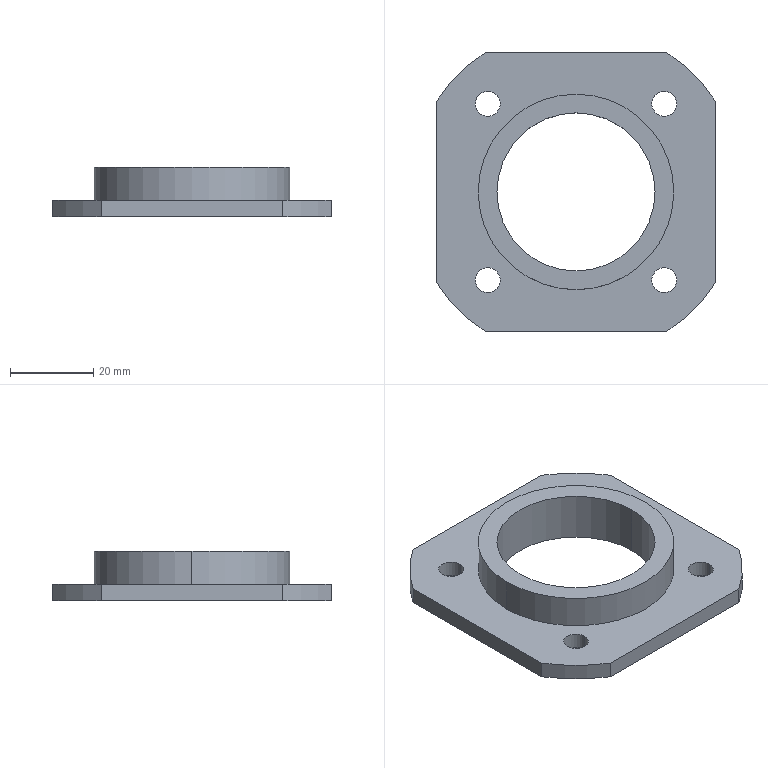Part | STEP file | Bearing cap | 1 solid | 23 faces | box 67 x 67 x 12 mm | volume 16840 mm3 | cylinder 16 | plane 7 | commonest cylinder face diameters 6 x8 80 x4 38 x2 47 x2
STEP:
#1=CARTESIAN_POINT('',(-18.213,21.213,0.));
#2=VERTEX_POINT('',#1);
#3=CARTESIAN_POINT('',(-24.213,21.213,0.));
#4=VERTEX_POINT('',#3);
#5=CARTESIAN_POINT('',(-21.213,21.213,0.));
#6=DIRECTION('',(0.,0.,-1.));
#7=DIRECTION('',(1.,0.,0.));
#8=AXIS2_PLACEMENT_3D('',#5,#6,#7);
#9=CIRCLE('',#8,3.);
#10=EDGE_CURVE('',#2,#4,#9,.T.);
#11=ORIENTED_EDGE('',*,*,#10,.F.);
#12=CARTESIAN_POINT('',(-18.213,21.213,-4.));
#13=VERTEX_POINT('',#12);
#14=CARTESIAN_POINT('',(-18.213,21.213,0.));
#15=DIRECTION('',(0.,0.,-1.));
#16=VECTOR('',#15,1000.);
#17=LINE('',#14,#16);
#18=EDGE_CURVE('',#2,#13,#17,.T.);
#19=ORIENTED_EDGE('',*,*,#18,.T.);
#20=CARTESIAN_POINT('',(-24.213,21.213,-4.));
#21=VERTEX_POINT('',#20);
#22=CARTESIAN_POINT('',(-21.213,21.213,-4.));
#23=DIRECTION('',(0.,0.,-1.));
#24=DIRECTION('',(1.,0.,0.));
#25=AXIS2_PLACEMENT_3D('',#22,#23,#24);
#26=CIRCLE('',#25,3.);
#27=EDGE_CURVE('',#13,#21,#26,.T.);
#28=ORIENTED_EDGE('',*,*,#27,.T.);
#29=CARTESIAN_POINT('',(-24.213,21.213,0.));
#30=DIRECTION('',(0.,0.,-1.));
#31=VECTOR('',#30,1000.);
#32=LINE('',#29,#31);
#33=EDGE_CURVE('',#4,#21,#32,.T.);
#34=ORIENTED_EDGE('',*,*,#33,.F.);
#35=EDGE_LOOP('',(#11,#19,#28,#34));
#36=FACE_OUTER_BOUND('',#35,.T.);
#37=CARTESIAN_POINT('',(-21.213,21.213,0.));
#38=DIRECTION('',(0.,0.,-1.));
#39=DIRECTION('',(-1.,0.,0.));
#40=AXIS2_PLACEMENT_3D('',#37,#38,#39);
#41=CYLINDRICAL_SURFACE('',#40,3.);
#42=ADVANCED_FACE('',(#36),#41,.F.);
#43=CARTESIAN_POINT('',(24.213,21.213,0.));
#44=VERTEX_POINT('',#43);
#45=CARTESIAN_POINT('',(18.213,21.213,0.));
#46=VERTEX_POINT('',#45);
#47=CARTESIAN_POINT('',(21.213,21.213,0.));
#48=DIRECTION('',(0.,0.,-1.));
#49=DIRECTION('',(0.,-1.,0.));
#50=AXIS2_PLACEMENT_3D('',#47,#48,#49);
#51=CIRCLE('',#50,3.);
#52=EDGE_CURVE('',#44,#46,#51,.T.);
#53=ORIENTED_EDGE('',*,*,#52,.F.);
#54=CARTESIAN_POINT('',(24.213,21.213,-4.));
#55=VERTEX_POINT('',#54);
#56=CARTESIAN_POINT('',(24.213,21.213,0.));
#57=DIRECTION('',(0.,0.,-1.));
#58=VECTOR('',#57,1000.);
#59=LINE('',#56,#58);
#60=EDGE_CURVE('',#44,#55,#59,.T.);
#61=ORIENTED_EDGE('',*,*,#60,.T.);
#62=CARTESIAN_POINT('',(18.213,21.213,-4.));
#63=VERTEX_POINT('',#62);
#64=CARTESIAN_POINT('',(21.213,21.213,-4.));
#65=DIRECTION('',(0.,0.,-1.));
#66=DIRECTION('',(0.,-1.,0.));
#67=AXIS2_PLACEMENT_3D('',#64,#65,#66);
#68=CIRCLE('',#67,3.);
#69=EDGE_CURVE('',#55,#63,#68,.T.);
#70=ORIENTED_EDGE('',*,*,#69,.T.);
#71=CARTESIAN_POINT('',(18.213,21.213,0.));
#72=DIRECTION('',(0.,0.,-1.));
#73=VECTOR('',#72,1000.);
#74=LINE('',#71,#73);
#75=EDGE_CURVE('',#46,#63,#74,.T.);
#76=ORIENTED_EDGE('',*,*,#75,.F.);
#77=EDGE_LOOP('',(#53,#61,#70,#76));
#78=FACE_OUTER_BOUND('',#77,.T.);
#79=CARTESIAN_POINT('',(21.213,21.213,0.));
#80=DIRECTION('',(0.,0.,-1.));
#81=DIRECTION('',(-1.,0.,0.));
#82=AXIS2_PLACEMENT_3D('',#79,#80,#81);
#83=CYLINDRICAL_SURFACE('',#82,3.);
#84=ADVANCED_FACE('',(#78),#83,.F.);
#85=CARTESIAN_POINT('',(-18.213,-21.213,0.));
#86=VERTEX_POINT('',#85);
#87=CARTESIAN_POINT('',(-24.213,-21.213,0.));
#88=VERTEX_POINT('',#87);
#89=CARTESIAN_POINT('',(-21.213,-21.213,0.));
#90=DIRECTION('',(0.,0.,-1.));
#91=DIRECTION('',(0.,1.,0.));
#92=AXIS2_PLACEMENT_3D('',#89,#90,#91);
#93=CIRCLE('',#92,3.);
#94=EDGE_CURVE('',#86,#88,#93,.T.);
#95=ORIENTED_EDGE('',*,*,#94,.F.);
#96=CARTESIAN_POINT('',(-18.213,-21.213,-4.));
#97=VERTEX_POINT('',#96);
#98=CARTESIAN_POINT('',(-18.213,-21.213,0.));
#99=DIRECTION('',(0.,0.,-1.));
#100=VECTOR('',#99,1000.);
#101=LINE('',#98,#100);
#102=EDGE_CURVE('',#86,#97,#101,.T.);
#103=ORIENTED_EDGE('',*,*,#102,.T.);
#104=CARTESIAN_POINT('',(-24.213,-21.213,-4.));
#105=VERTEX_POINT('',#104);
#106=CARTESIAN_POINT('',(-21.213,-21.213,-4.));
#107=DIRECTION('',(0.,0.,-1.));
#108=DIRECTION('',(0.,1.,0.));
#109=AXIS2_PLACEMENT_3D('',#106,#107,#108);
#110=CIRCLE('',#109,3.);
#111=EDGE_CURVE('',#97,#105,#110,.T.);
#112=ORIENTED_EDGE('',*,*,#111,.T.);
#113=CARTESIAN_POINT('',(-24.213,-21.213,0.));
#114=DIRECTION('',(0.,0.,-1.));
#115=VECTOR('',#114,1000.);
#116=LINE('',#113,#115);
#117=EDGE_CURVE('',#88,#105,#116,.T.);
#118=ORIENTED_EDGE('',*,*,#117,.F.);
#119=EDGE_LOOP('',(#95,#103,#112,#118));
#120=FACE_OUTER_BOUND('',#119,.T.);
#121=CARTESIAN_POINT('',(-21.213,-21.213,0.));
#122=DIRECTION('',(0.,0.,-1.));
#123=DIRECTION('',(-1.,0.,0.));
#124=AXIS2_PLACEMENT_3D('',#121,#122,#123);
#125=CYLINDRICAL_SURFACE('',#124,3.);
#126=ADVANCED_FACE('',(#120),#125,.F.);
#127=CARTESIAN_POINT('',(24.213,-21.213,0.));
#128=VERTEX_POINT('',#127);
#129=CARTESIAN_POINT('',(18.213,-21.213,0.));
#130=VERTEX_POINT('',#129);
#131=CARTESIAN_POINT('',(21.213,-21.213,0.));
#132=DIRECTION('',(0.,0.,-1.));
#133=DIRECTION('',(-1.,0.,0.));
#134=AXIS2_PLACEMENT_3D('',#131,#132,#133);
#135=CIRCLE('',#134,3.);
#136=EDGE_CURVE('',#128,#130,#135,.T.);
#137=ORIENTED_EDGE('',*,*,#136,.F.);
#138=CARTESIAN_POINT('',(24.213,-21.213,-4.));
#139=VERTEX_POINT('',#138);
#140=CARTESIAN_POINT('',(24.213,-21.213,0.));
#141=DIRECTION('',(0.,0.,-1.));
#142=VECTOR('',#141,1000.);
#143=LINE('',#140,#142);
#144=EDGE_CURVE('',#128,#139,#143,.T.);
#145=ORIENTED_EDGE('',*,*,#144,.T.);
#146=CARTESIAN_POINT('',(18.213,-21.213,-4.));
#147=VERTEX_POINT('',#146);
#148=CARTESIAN_POINT('',(21.213,-21.213,-4.));
#149=DIRECTION('',(0.,0.,-1.));
#150=DIRECTION('',(-1.,0.,0.));
#151=AXIS2_PLACEMENT_3D('',#148,#149,#150);
#152=CIRCLE('',#151,3.);
#153=EDGE_CURVE('',#139,#147,#152,.T.);
#154=ORIENTED_EDGE('',*,*,#153,.T.);
#155=CARTESIAN_POINT('',(18.213,-21.213,0.));
#156=DIRECTION('',(0.,0.,-1.));
#157=VECTOR('',#156,1000.);
#158=LINE('',#155,#157);
#159=EDGE_CURVE('',#130,#147,#158,.T.);
#160=ORIENTED_EDGE('',*,*,#159,.F.);
#161=EDGE_LOOP('',(#137,#145,#154,#160));
#162=FACE_OUTER_BOUND('',#161,.T.);
#163=CARTESIAN_POINT('',(21.213,-21.213,0.));
#164=DIRECTION('',(0.,0.,-1.));
#165=DIRECTION('',(-1.,0.,0.));
#166=AXIS2_PLACEMENT_3D('',#163,#164,#165);
#167=CYLINDRICAL_SURFACE('',#166,3.);
#168=ADVANCED_FACE('',(#162),#167,.F.);
#169=CARTESIAN_POINT('',(-19.,0.,8.));
#170=VERTEX_POINT('',#169);
#171=CARTESIAN_POINT('',(19.,0.,8.));
#172=VERTEX_POINT('',#171);
#173=CARTESIAN_POINT('',(0.,0.,8.));
#174=DIRECTION('',(0.,0.,1.));
#175=DIRECTION('',(1.,0.,0.));
#176=AXIS2_PLACEMENT_3D('',#173,#174,#175);
#177=CIRCLE('',#176,19.);
#178=EDGE_CURVE('',#170,#172,#177,.T.);
#179=ORIENTED_EDGE('',*,*,#178,.T.);
#180=CARTESIAN_POINT('',(19.,0.,-4.));
#181=VERTEX_POINT('',#180);
#182=CARTESIAN_POINT('',(19.,0.,8.));
#183=DIRECTION('',(0.,0.,-1.));
#184=VECTOR('',#183,1000.);
#185=LINE('',#182,#184);
#186=EDGE_CURVE('',#172,#181,#185,.T.);
#187=ORIENTED_EDGE('',*,*,#186,.T.);
#188=CARTESIAN_POINT('',(-19.,0.,-4.));
#189=VERTEX_POINT('',#188);
#190=CARTESIAN_POINT('',(0.,0.,-4.));
#191=DIRECTION('',(0.,0.,1.));
#192=DIRECTION('',(-1.,0.,0.));
#193=AXIS2_PLACEMENT_3D('',#190,#191,#192);
#194=CIRCLE('',#193,19.);
#195=EDGE_CURVE('',#189,#181,#194,.T.);
#196=ORIENTED_EDGE('',*,*,#195,.F.);
#197=CARTESIAN_POINT('',(-19.,0.,8.));
#198=DIRECTION('',(0.,0.,-1.));
#199=VECTOR('',#198,1000.);
#200=LINE('',#197,#199);
#201=EDGE_CURVE('',#170,#189,#200,.T.);
#202=ORIENTED_EDGE('',*,*,#201,.F.);
#203=EDGE_LOOP('',(#179,#187,#196,#202));
#204=FACE_OUTER_BOUND('',#203,.T.);
#205=CARTESIAN_POINT('',(0.,0.,8.));
#206=DIRECTION('',(0.,0.,-1.));
#207=DIRECTION('',(-1.,0.,0.));
#208=AXIS2_PLACEMENT_3D('',#205,#206,#207);
#209=CYLINDRICAL_SURFACE('',#208,19.);
#210=ADVANCED_FACE('',(#204),#209,.F.);
#211=CARTESIAN_POINT('',(23.5,0.,8.));
#212=VERTEX_POINT('',#211);
#213=CARTESIAN_POINT('',(-23.5,0.,8.));
#214=VERTEX_POINT('',#213);
#215=CARTESIAN_POINT('',(0.,0.,8.));
#216=DIRECTION('',(0.,0.,1.));
#217=DIRECTION('',(1.,0.,0.));
#218=AXIS2_PLACEMENT_3D('',#215,#216,#217);
#219=CIRCLE('',#218,23.5);
#220=EDGE_CURVE('',#212,#214,#219,.T.);
#221=ORIENTED_EDGE('',*,*,#220,.F.);
#222=CARTESIAN_POINT('',(23.5,0.,0.));
#223=VERTEX_POINT('',#222);
#224=CARTESIAN_POINT('',(23.5,0.,8.));
#225=DIRECTION('',(0.,0.,-1.));
#226=VECTOR('',#225,1000.);
#227=LINE('',#224,#226);
#228=EDGE_CURVE('',#212,#223,#227,.T.);
#229=ORIENTED_EDGE('',*,*,#228,.T.);
#230=CARTESIAN_POINT('',(-23.5,0.,0.));
#231=VERTEX_POINT('',#230);
#232=CARTESIAN_POINT('',(0.,0.,0.));
#233=DIRECTION('',(0.,0.,-1.));
#234=DIRECTION('',(-1.,0.,0.));
#235=AXIS2_PLACEMENT_3D('',#232,#233,#234);
#236=CIRCLE('',#235,23.5);
#237=EDGE_CURVE('',#231,#223,#236,.T.);
#238=ORIENTED_EDGE('',*,*,#237,.F.);
#239=CARTESIAN_POINT('',(-23.5,0.,8.));
#240=DIRECTION('',(0.,0.,-1.));
#241=VECTOR('',#240,1000.);
#242=LINE('',#239,#241);
#243=EDGE_CURVE('',#214,#231,#242,.T.);
#244=ORIENTED_EDGE('',*,*,#243,.F.);
#245=EDGE_LOOP('',(#221,#229,#238,#244));
#246=FACE_OUTER_BOUND('',#245,.T.);
#247=CARTESIAN_POINT('',(0.,0.,8.));
#248=DIRECTION('',(0.,0.,-1.));
#249=DIRECTION('',(-1.,0.,0.));
#250=AXIS2_PLACEMENT_3D('',#247,#248,#249);
#251=CYLINDRICAL_SURFACE('',#250,23.5);
#252=ADVANCED_FACE('',(#246),#251,.T.);
#253=CARTESIAN_POINT('',(0.,0.,8.));
#254=DIRECTION('',(0.,0.,1.));
#255=DIRECTION('',(1.,0.,0.));
#256=AXIS2_PLACEMENT_3D('',#253,#254,#255);
#257=CIRCLE('',#256,23.5);
#258=EDGE_CURVE('',#214,#212,#257,.T.);
#259=ORIENTED_EDGE('',*,*,#258,.T.);
#260=ORIENTED_EDGE('',*,*,#220,.T.);
#261=EDGE_LOOP('',(#259,#260));
#262=FACE_OUTER_BOUND('',#261,.T.);
#263=ORIENTED_EDGE('',*,*,#178,.F.);
#264=CARTESIAN_POINT('',(0.,0.,8.));
#265=DIRECTION('',(0.,0.,1.));
#266=DIRECTION('',(1.,0.,0.));
#267=AXIS2_PLACEMENT_3D('',#264,#265,#266);
#268=CIRCLE('',#267,19.);
#269=EDGE_CURVE('',#172,#170,#268,.T.);
#270=ORIENTED_EDGE('',*,*,#269,.F.);
#271=EDGE_LOOP('',(#263,#270));
#272=FACE_BOUND('',#271,.T.);
#273=CARTESIAN_POINT('',(0.,0.,8.));
#274=DIRECTION('',(0.,0.,1.));
#275=DIRECTION('',(1.,0.,0.));
#276=AXIS2_PLACEMENT_3D('',#273,#274,#275);
#277=PLANE('',#276);
#278=ADVANCED_FACE('',(#262,#272),#277,.T.);
#279=ORIENTED_EDGE('',*,*,#228,.F.);
#280=ORIENTED_EDGE('',*,*,#258,.F.);
#281=ORIENTED_EDGE('',*,*,#243,.T.);
#282=CARTESIAN_POINT('',(0.,0.,0.));
#283=DIRECTION('',(0.,0.,-1.));
#284=DIRECTION('',(-1.,0.,0.));
#285=AXIS2_PLACEMENT_3D('',#282,#283,#284);
#286=CIRCLE('',#285,23.5);
#287=EDGE_CURVE('',#223,#231,#286,.T.);
#288=ORIENTED_EDGE('',*,*,#287,.F.);
#289=EDGE_LOOP('',(#279,#280,#281,#288));
#290=FACE_OUTER_BOUND('',#289,.T.);
#291=CARTESIAN_POINT('',(0.,0.,8.));
#292=DIRECTION('',(0.,0.,-1.));
#293=DIRECTION('',(-1.,0.,0.));
#294=AXIS2_PLACEMENT_3D('',#291,#292,#293);
#295=CYLINDRICAL_SURFACE('',#294,23.5);
#296=ADVANCED_FACE('',(#290),#295,.T.);
#297=ORIENTED_EDGE('',*,*,#186,.F.);
#298=ORIENTED_EDGE('',*,*,#269,.T.);
#299=ORIENTED_EDGE('',*,*,#201,.T.);
#300=CARTESIAN_POINT('',(0.,0.,-4.));
#301=DIRECTION('',(0.,0.,1.));
#302=DIRECTION('',(-1.,0.,0.));
#303=AXIS2_PLACEMENT_3D('',#300,#301,#302);
#304=CIRCLE('',#303,19.);
#305=EDGE_CURVE('',#181,#189,#304,.T.);
#306=ORIENTED_EDGE('',*,*,#305,.F.);
#307=EDGE_LOOP('',(#297,#298,#299,#306));
#308=FACE_OUTER_BOUND('',#307,.T.);
#309=CARTESIAN_POINT('',(0.,0.,8.));
#310=DIRECTION('',(0.,0.,-1.));
#311=DIRECTION('',(-1.,0.,0.));
#312=AXIS2_PLACEMENT_3D('',#309,#310,#311);
#313=CYLINDRICAL_SURFACE('',#312,19.);
#314=ADVANCED_FACE('',(#308),#313,.F.);
#315=CARTESIAN_POINT('',(-21.213,21.213,0.));
#316=DIRECTION('',(0.,0.,-1.));
#317=DIRECTION('',(1.,0.,0.));
#318=AXIS2_PLACEMENT_3D('',#315,#316,#317);
#319=CIRCLE('',#318,3.);
#320=EDGE_CURVE('',#4,#2,#319,.T.);
#321=ORIENTED_EDGE('',*,*,#320,.T.);
#322=ORIENTED_EDGE('',*,*,#10,.T.);
#323=EDGE_LOOP('',(#321,#322));
#324=FACE_BOUND('',#323,.T.);
#325=CARTESIAN_POINT('',(21.213,21.213,0.));
#326=DIRECTION('',(0.,0.,-1.));
#327=DIRECTION('',(0.,-1.,0.));
#328=AXIS2_PLACEMENT_3D('',#325,#326,#327);
#329=CIRCLE('',#328,3.);
#330=EDGE_CURVE('',#46,#44,#329,.T.);
#331=ORIENTED_EDGE('',*,*,#330,.T.);
#332=ORIENTED_EDGE('',*,*,#52,.T.);
#333=EDGE_LOOP('',(#331,#332));
#334=FACE_BOUND('',#333,.T.);
#335=CARTESIAN_POINT('',(-21.213,-21.213,0.));
#336=DIRECTION('',(0.,0.,-1.));
#337=DIRECTION('',(0.,1.,0.));
#338=AXIS2_PLACEMENT_3D('',#335,#336,#337);
#339=CIRCLE('',#338,3.);
#340=EDGE_CURVE('',#88,#86,#339,.T.);
#341=ORIENTED_EDGE('',*,*,#340,.T.);
#342=ORIENTED_EDGE('',*,*,#94,.T.);
#343=EDGE_LOOP('',(#341,#342));
#344=FACE_BOUND('',#343,.T.);
#345=CARTESIAN_POINT('',(21.213,-21.213,0.));
#346=DIRECTION('',(0.,0.,-1.));
#347=DIRECTION('',(-1.,0.,0.));
#348=AXIS2_PLACEMENT_3D('',#345,#346,#347);
#349=CIRCLE('',#348,3.);
#350=EDGE_CURVE('',#130,#128,#349,.T.);
#351=ORIENTED_EDGE('',*,*,#350,.T.);
#352=ORIENTED_EDGE('',*,*,#136,.T.);
#353=EDGE_LOOP('',(#351,#352));
#354=FACE_BOUND('',#353,.T.);
#355=CARTESIAN_POINT('',(33.5,21.857,0.));
#356=VERTEX_POINT('',#355);
#357=CARTESIAN_POINT('',(33.5,-21.857,0.));
#358=VERTEX_POINT('',#357);
#359=CARTESIAN_POINT('',(33.5,0.,0.));
#360=DIRECTION('',(0.,-1.,0.));
#361=VECTOR('',#360,1000.);
#362=LINE('',#359,#361);
#363=EDGE_CURVE('',#356,#358,#362,.T.);
#364=ORIENTED_EDGE('',*,*,#363,.F.);
#365=CARTESIAN_POINT('',(21.857,33.5,0.));
#366=VERTEX_POINT('',#365);
#367=CARTESIAN_POINT('',(0.,0.,0.));
#368=DIRECTION('',(0.,0.,-1.));
#369=DIRECTION('',(-1.,0.,0.));
#370=AXIS2_PLACEMENT_3D('',#367,#368,#369);
#371=CIRCLE('',#370,40.);
#372=EDGE_CURVE('',#366,#356,#371,.T.);
#373=ORIENTED_EDGE('',*,*,#372,.F.);
#374=CARTESIAN_POINT('',(-21.857,33.5,0.));
#375=VERTEX_POINT('',#374);
#376=CARTESIAN_POINT('',(0.,33.5,0.));
#377=DIRECTION('',(1.,0.,0.));
#378=VECTOR('',#377,1000.);
#379=LINE('',#376,#378);
#380=EDGE_CURVE('',#375,#366,#379,.T.);
#381=ORIENTED_EDGE('',*,*,#380,.F.);
#382=CARTESIAN_POINT('',(-33.5,21.857,0.));
#383=VERTEX_POINT('',#382);
#384=CARTESIAN_POINT('',(0.,0.,0.));
#385=DIRECTION('',(0.,0.,-1.));
#386=DIRECTION('',(-1.,0.,0.));
#387=AXIS2_PLACEMENT_3D('',#384,#385,#386);
#388=CIRCLE('',#387,40.);
#389=EDGE_CURVE('',#383,#375,#388,.T.);
#390=ORIENTED_EDGE('',*,*,#389,.F.);
#391=CARTESIAN_POINT('',(-33.5,-21.857,0.));
#392=VERTEX_POINT('',#391);
#393=CARTESIAN_POINT('',(-33.5,0.,0.));
#394=DIRECTION('',(0.,1.,0.));
#395=VECTOR('',#394,1000.);
#396=LINE('',#393,#395);
#397=EDGE_CURVE('',#392,#383,#396,.T.);
#398=ORIENTED_EDGE('',*,*,#397,.F.);
#399=CARTESIAN_POINT('',(-21.857,-33.5,0.));
#400=VERTEX_POINT('',#399);
#401=CARTESIAN_POINT('',(0.,0.,0.));
#402=DIRECTION('',(0.,0.,-1.));
#403=DIRECTION('',(-1.,0.,0.));
#404=AXIS2_PLACEMENT_3D('',#401,#402,#403);
#405=CIRCLE('',#404,40.);
#406=EDGE_CURVE('',#400,#392,#405,.T.);
#407=ORIENTED_EDGE('',*,*,#406,.F.);
#408=CARTESIAN_POINT('',(21.857,-33.5,0.));
#409=VERTEX_POINT('',#408);
#410=CARTESIAN_POINT('',(0.,-33.5,0.));
#411=DIRECTION('',(-1.,0.,0.));
#412=VECTOR('',#411,1000.);
#413=LINE('',#410,#412);
#414=EDGE_CURVE('',#409,#400,#413,.T.);
#415=ORIENTED_EDGE('',*,*,#414,.F.);
#416=CARTESIAN_POINT('',(0.,0.,0.));
#417=DIRECTION('',(0.,0.,-1.));
#418=DIRECTION('',(-1.,0.,0.));
#419=AXIS2_PLACEMENT_3D('',#416,#417,#418);
#420=CIRCLE('',#419,40.);
#421=EDGE_CURVE('',#358,#409,#420,.T.);
#422=ORIENTED_EDGE('',*,*,#421,.F.);
#423=EDGE_LOOP('',(#364,#373,#381,#390,#398,#407,#415,#422));
#424=FACE_OUTER_BOUND('',#423,.T.);
#425=ORIENTED_EDGE('',*,*,#237,.T.);
#426=ORIENTED_EDGE('',*,*,#287,.T.);
#427=EDGE_LOOP('',(#425,#426));
#428=FACE_BOUND('',#427,.T.);
#429=CARTESIAN_POINT('',(0.,0.,0.));
#430=DIRECTION('',(0.,0.,-1.));
#431=DIRECTION('',(-1.,0.,0.));
#432=AXIS2_PLACEMENT_3D('',#429,#430,#431);
#433=PLANE('',#432);
#434=ADVANCED_FACE('',(#324,#334,#344,#354,#424,#428),#433,.F.);
#435=ORIENTED_EDGE('',*,*,#363,.T.);
#436=CARTESIAN_POINT('',(33.5,-21.857,-4.));
#437=VERTEX_POINT('',#436);
#438=CARTESIAN_POINT('',(33.5,-21.857,-4.));
#439=DIRECTION('',(0.,0.,1.));
#440=VECTOR('',#439,1000.);
#441=LINE('',#438,#440);
#442=EDGE_CURVE('',#437,#358,#441,.T.);
#443=ORIENTED_EDGE('',*,*,#442,.F.);
#444=CARTESIAN_POINT('',(33.5,21.857,-4.));
#445=VERTEX_POINT('',#444);
#446=CARTESIAN_POINT('',(33.5,0.,-4.));
#447=DIRECTION('',(0.,-1.,0.));
#448=VECTOR('',#447,1000.);
#449=LINE('',#446,#448);
#450=EDGE_CURVE('',#445,#437,#449,.T.);
#451=ORIENTED_EDGE('',*,*,#450,.F.);
#452=CARTESIAN_POINT('',(33.5,21.857,-4.));
#453=DIRECTION('',(0.,0.,1.));
#454=VECTOR('',#453,1000.);
#455=LINE('',#452,#454);
#456=EDGE_CURVE('',#445,#356,#455,.T.);
#457=ORIENTED_EDGE('',*,*,#456,.T.);
#458=EDGE_LOOP('',(#435,#443,#451,#457));
#459=FACE_OUTER_BOUND('',#458,.T.);
#460=CARTESIAN_POINT('',(33.5,0.,-4.));
#461=DIRECTION('',(-1.,0.,0.));
#462=DIRECTION('',(0.,-1.,0.));
#463=AXIS2_PLACEMENT_3D('',#460,#461,#462);
#464=PLANE('',#463);
#465=ADVANCED_FACE('',(#459),#464,.F.);
#466=ORIENTED_EDGE('',*,*,#421,.T.);
#467=CARTESIAN_POINT('',(21.857,-33.5,-4.));
#468=VERTEX_POINT('',#467);
#469=CARTESIAN_POINT('',(21.857,-33.5,-4.));
#470=DIRECTION('',(0.,0.,1.));
#471=VECTOR('',#470,1000.);
#472=LINE('',#469,#471);
#473=EDGE_CURVE('',#468,#409,#472,.T.);
#474=ORIENTED_EDGE('',*,*,#473,.F.);
#475=CARTESIAN_POINT('',(0.,0.,-4.));
#476=DIRECTION('',(0.,0.,-1.));
#477=DIRECTION('',(-1.,0.,0.));
#478=AXIS2_PLACEMENT_3D('',#475,#476,#477);
#479=CIRCLE('',#478,40.);
#480=EDGE_CURVE('',#437,#468,#479,.T.);
#481=ORIENTED_EDGE('',*,*,#480,.F.);
#482=ORIENTED_EDGE('',*,*,#442,.T.);
#483=EDGE_LOOP('',(#466,#474,#481,#482));
#484=FACE_OUTER_BOUND('',#483,.T.);
#485=CARTESIAN_POINT('',(0.,0.,-4.));
#486=DIRECTION('',(0.,0.,1.));
#487=DIRECTION('',(1.,0.,0.));
#488=AXIS2_PLACEMENT_3D('',#485,#486,#487);
#489=CYLINDRICAL_SURFACE('',#488,40.);
#490=ADVANCED_FACE('',(#484),#489,.T.);
#491=ORIENTED_EDGE('',*,*,#414,.T.);
#492=CARTESIAN_POINT('',(-21.857,-33.5,-4.));
#493=VERTEX_POINT('',#492);
#494=CARTESIAN_POINT('',(-21.857,-33.5,-4.));
#495=DIRECTION('',(0.,0.,1.));
#496=VECTOR('',#495,1000.);
#497=LINE('',#494,#496);
#498=EDGE_CURVE('',#493,#400,#497,.T.);
#499=ORIENTED_EDGE('',*,*,#498,.F.);
#500=CARTESIAN_POINT('',(0.,-33.5,-4.));
#501=DIRECTION('',(-1.,0.,0.));
#502=VECTOR('',#501,1000.);
#503=LINE('',#500,#502);
#504=EDGE_CURVE('',#468,#493,#503,.T.);
#505=ORIENTED_EDGE('',*,*,#504,.F.);
#506=ORIENTED_EDGE('',*,*,#473,.T.);
#507=EDGE_LOOP('',(#491,#499,#505,#506));
#508=FACE_OUTER_BOUND('',#507,.T.);
#509=CARTESIAN_POINT('',(0.,-33.5,-4.));
#510=DIRECTION('',(0.,1.,0.));
#511=DIRECTION('',(-1.,0.,0.));
#512=AXIS2_PLACEMENT_3D('',#509,#510,#511);
#513=PLANE('',#512);
#514=ADVANCED_FACE('',(#508),#513,.F.);
#515=ORIENTED_EDGE('',*,*,#406,.T.);
#516=CARTESIAN_POINT('',(-33.5,-21.857,-4.));
#517=VERTEX_POINT('',#516);
#518=CARTESIAN_POINT('',(-33.5,-21.857,-4.));
#519=DIRECTION('',(0.,0.,1.));
#520=VECTOR('',#519,1000.);
#521=LINE('',#518,#520);
#522=EDGE_CURVE('',#517,#392,#521,.T.);
#523=ORIENTED_EDGE('',*,*,#522,.F.);
#524=CARTESIAN_POINT('',(0.,0.,-4.));
#525=DIRECTION('',(0.,0.,-1.));
#526=DIRECTION('',(-1.,0.,0.));
#527=AXIS2_PLACEMENT_3D('',#524,#525,#526);
#528=CIRCLE('',#527,40.);
#529=EDGE_CURVE('',#493,#517,#528,.T.);
#530=ORIENTED_EDGE('',*,*,#529,.F.);
#531=ORIENTED_EDGE('',*,*,#498,.T.);
#532=EDGE_LOOP('',(#515,#523,#530,#531));
#533=FACE_OUTER_BOUND('',#532,.T.);
#534=CARTESIAN_POINT('',(0.,0.,-4.));
#535=DIRECTION('',(0.,0.,1.));
#536=DIRECTION('',(1.,0.,0.));
#537=AXIS2_PLACEMENT_3D('',#534,#535,#536);
#538=CYLINDRICAL_SURFACE('',#537,40.);
#539=ADVANCED_FACE('',(#533),#538,.T.);
#540=ORIENTED_EDGE('',*,*,#397,.T.);
#541=CARTESIAN_POINT('',(-33.5,21.857,-4.));
#542=VERTEX_POINT('',#541);
#543=CARTESIAN_POINT('',(-33.5,21.857,-4.));
#544=DIRECTION('',(0.,0.,1.));
#545=VECTOR('',#544,1000.);
#546=LINE('',#543,#545);
#547=EDGE_CURVE('',#542,#383,#546,.T.);
#548=ORIENTED_EDGE('',*,*,#547,.F.);
#549=CARTESIAN_POINT('',(-33.5,0.,-4.));
#550=DIRECTION('',(0.,1.,0.));
#551=VECTOR('',#550,1000.);
#552=LINE('',#549,#551);
#553=EDGE_CURVE('',#517,#542,#552,.T.);
#554=ORIENTED_EDGE('',*,*,#553,.F.);
#555=ORIENTED_EDGE('',*,*,#522,.T.);
#556=EDGE_LOOP('',(#540,#548,#554,#555));
#557=FACE_OUTER_BOUND('',#556,.T.);
#558=CARTESIAN_POINT('',(-33.5,0.,-4.));
#559=DIRECTION('',(1.,0.,0.));
#560=DIRECTION('',(0.,1.,0.));
#561=AXIS2_PLACEMENT_3D('',#558,#559,#560);
#562=PLANE('',#561);
#563=ADVANCED_FACE('',(#557),#562,.F.);
#564=ORIENTED_EDGE('',*,*,#389,.T.);
#565=CARTESIAN_POINT('',(-21.857,33.5,-4.));
#566=VERTEX_POINT('',#565);
#567=CARTESIAN_POINT('',(-21.857,33.5,-4.));
#568=DIRECTION('',(0.,0.,1.));
#569=VECTOR('',#568,1000.);
#570=LINE('',#567,#569);
#571=EDGE_CURVE('',#566,#375,#570,.T.);
#572=ORIENTED_EDGE('',*,*,#571,.F.);
#573=CARTESIAN_POINT('',(0.,0.,-4.));
#574=DIRECTION('',(0.,0.,-1.));
#575=DIRECTION('',(-1.,0.,0.));
#576=AXIS2_PLACEMENT_3D('',#573,#574,#575);
#577=CIRCLE('',#576,40.);
#578=EDGE_CURVE('',#542,#566,#577,.T.);
#579=ORIENTED_EDGE('',*,*,#578,.F.);
#580=ORIENTED_EDGE('',*,*,#547,.T.);
#581=EDGE_LOOP('',(#564,#572,#579,#580));
#582=FACE_OUTER_BOUND('',#581,.T.);
#583=CARTESIAN_POINT('',(0.,0.,-4.));
#584=DIRECTION('',(0.,0.,1.));
#585=DIRECTION('',(1.,0.,0.));
#586=AXIS2_PLACEMENT_3D('',#583,#584,#585);
#587=CYLINDRICAL_SURFACE('',#586,40.);
#588=ADVANCED_FACE('',(#582),#587,.T.);
#589=ORIENTED_EDGE('',*,*,#380,.T.);
#590=CARTESIAN_POINT('',(21.857,33.5,-4.));
#591=VERTEX_POINT('',#590);
#592=CARTESIAN_POINT('',(21.857,33.5,-4.));
#593=DIRECTION('',(0.,0.,1.));
#594=VECTOR('',#593,1000.);
#595=LINE('',#592,#594);
#596=EDGE_CURVE('',#591,#366,#595,.T.);
#597=ORIENTED_EDGE('',*,*,#596,.F.);
#598=CARTESIAN_POINT('',(0.,33.5,-4.));
#599=DIRECTION('',(1.,0.,0.));
#600=VECTOR('',#599,1000.);
#601=LINE('',#598,#600);
#602=EDGE_CURVE('',#566,#591,#601,.T.);
#603=ORIENTED_EDGE('',*,*,#602,.F.);
#604=ORIENTED_EDGE('',*,*,#571,.T.);
#605=EDGE_LOOP('',(#589,#597,#603,#604));
#606=FACE_OUTER_BOUND('',#605,.T.);
#607=CARTESIAN_POINT('',(0.,33.5,-4.));
#608=DIRECTION('',(0.,-1.,0.));
#609=DIRECTION('',(1.,0.,0.));
#610=AXIS2_PLACEMENT_3D('',#607,#608,#609);
#611=PLANE('',#610);
#612=ADVANCED_FACE('',(#606),#611,.F.);
#613=ORIENTED_EDGE('',*,*,#372,.T.);
#614=ORIENTED_EDGE('',*,*,#456,.F.);
#615=CARTESIAN_POINT('',(0.,0.,-4.));
#616=DIRECTION('',(0.,0.,-1.));
#617=DIRECTION('',(-1.,0.,0.));
#618=AXIS2_PLACEMENT_3D('',#615,#616,#617);
#619=CIRCLE('',#618,40.);
#620=EDGE_CURVE('',#591,#445,#619,.T.);
#621=ORIENTED_EDGE('',*,*,#620,.F.);
#622=ORIENTED_EDGE('',*,*,#596,.T.);
#623=EDGE_LOOP('',(#613,#614,#621,#622));
#624=FACE_OUTER_BOUND('',#623,.T.);
#625=CARTESIAN_POINT('',(0.,0.,-4.));
#626=DIRECTION('',(0.,0.,1.));
#627=DIRECTION('',(1.,0.,0.));
#628=AXIS2_PLACEMENT_3D('',#625,#626,#627);
#629=CYLINDRICAL_SURFACE('',#628,40.);
#630=ADVANCED_FACE('',(#624),#629,.T.);
#631=CARTESIAN_POINT('',(-21.213,21.213,-4.));
#632=DIRECTION('',(0.,0.,-1.));
#633=DIRECTION('',(1.,0.,0.));
#634=AXIS2_PLACEMENT_3D('',#631,#632,#633);
#635=CIRCLE('',#634,3.);
#636=EDGE_CURVE('',#21,#13,#635,.T.);
#637=ORIENTED_EDGE('',*,*,#636,.F.);
#638=ORIENTED_EDGE('',*,*,#27,.F.);
#639=EDGE_LOOP('',(#637,#638));
#640=FACE_BOUND('',#639,.T.);
#641=CARTESIAN_POINT('',(21.213,21.213,-4.));
#642=DIRECTION('',(0.,0.,-1.));
#643=DIRECTION('',(0.,-1.,0.));
#644=AXIS2_PLACEMENT_3D('',#641,#642,#643);
#645=CIRCLE('',#644,3.);
#646=EDGE_CURVE('',#63,#55,#645,.T.);
#647=ORIENTED_EDGE('',*,*,#646,.F.);
#648=ORIENTED_EDGE('',*,*,#69,.F.);
#649=EDGE_LOOP('',(#647,#648));
#650=FACE_BOUND('',#649,.T.);
#651=CARTESIAN_POINT('',(-21.213,-21.213,-4.));
#652=DIRECTION('',(0.,0.,-1.));
#653=DIRECTION('',(0.,1.,0.));
#654=AXIS2_PLACEMENT_3D('',#651,#652,#653);
#655=CIRCLE('',#654,3.);
#656=EDGE_CURVE('',#105,#97,#655,.T.);
#657=ORIENTED_EDGE('',*,*,#656,.F.);
#658=ORIENTED_EDGE('',*,*,#111,.F.);
#659=EDGE_LOOP('',(#657,#658));
#660=FACE_BOUND('',#659,.T.);
#661=CARTESIAN_POINT('',(21.213,-21.213,-4.));
#662=DIRECTION('',(0.,0.,-1.));
#663=DIRECTION('',(-1.,0.,0.));
#664=AXIS2_PLACEMENT_3D('',#661,#662,#663);
#665=CIRCLE('',#664,3.);
#666=EDGE_CURVE('',#147,#139,#665,.T.);
#667=ORIENTED_EDGE('',*,*,#666,.F.);
#668=ORIENTED_EDGE('',*,*,#153,.F.);
#669=EDGE_LOOP('',(#667,#668));
#670=FACE_BOUND('',#669,.T.);
#671=ORIENTED_EDGE('',*,*,#450,.T.);
#672=ORIENTED_EDGE('',*,*,#480,.T.);
#673=ORIENTED_EDGE('',*,*,#504,.T.);
#674=ORIENTED_EDGE('',*,*,#529,.T.);
#675=ORIENTED_EDGE('',*,*,#553,.T.);
#676=ORIENTED_EDGE('',*,*,#578,.T.);
#677=ORIENTED_EDGE('',*,*,#602,.T.);
#678=ORIENTED_EDGE('',*,*,#620,.T.);
#679=EDGE_LOOP('',(#671,#672,#673,#674,#675,#676,#677,#678));
#680=FACE_OUTER_BOUND('',#679,.T.);
#681=ORIENTED_EDGE('',*,*,#195,.T.);
#682=ORIENTED_EDGE('',*,*,#305,.T.);
#683=EDGE_LOOP('',(#681,#682));
#684=FACE_BOUND('',#683,.T.);
#685=CARTESIAN_POINT('',(0.,0.,-4.));
#686=DIRECTION('',(0.,0.,-1.));
#687=DIRECTION('',(-1.,0.,0.));
#688=AXIS2_PLACEMENT_3D('',#685,#686,#687);
#689=PLANE('',#688);
#690=ADVANCED_FACE('',(#640,#650,#660,#670,#680,#684),#689,.T.);
#691=ORIENTED_EDGE('',*,*,#144,.F.);
#692=ORIENTED_EDGE('',*,*,#350,.F.);
#693=ORIENTED_EDGE('',*,*,#159,.T.);
#694=ORIENTED_EDGE('',*,*,#666,.T.);
#695=EDGE_LOOP('',(#691,#692,#693,#694));
#696=FACE_OUTER_BOUND('',#695,.T.);
#697=CARTESIAN_POINT('',(21.213,-21.213,0.));
#698=DIRECTION('',(0.,0.,-1.));
#699=DIRECTION('',(-1.,0.,0.));
#700=AXIS2_PLACEMENT_3D('',#697,#698,#699);
#701=CYLINDRICAL_SURFACE('',#700,3.);
#702=ADVANCED_FACE('',(#696),#701,.F.);
#703=ORIENTED_EDGE('',*,*,#102,.F.);
#704=ORIENTED_EDGE('',*,*,#340,.F.);
#705=ORIENTED_EDGE('',*,*,#117,.T.);
#706=ORIENTED_EDGE('',*,*,#656,.T.);
#707=EDGE_LOOP('',(#703,#704,#705,#706));
#708=FACE_OUTER_BOUND('',#707,.T.);
#709=CARTESIAN_POINT('',(-21.213,-21.213,0.));
#710=DIRECTION('',(0.,0.,-1.));
#711=DIRECTION('',(-1.,0.,0.));
#712=AXIS2_PLACEMENT_3D('',#709,#710,#711);
#713=CYLINDRICAL_SURFACE('',#712,3.);
#714=ADVANCED_FACE('',(#708),#713,.F.);
#715=ORIENTED_EDGE('',*,*,#60,.F.);
#716=ORIENTED_EDGE('',*,*,#330,.F.);
#717=ORIENTED_EDGE('',*,*,#75,.T.);
#718=ORIENTED_EDGE('',*,*,#646,.T.);
#719=EDGE_LOOP('',(#715,#716,#717,#718));
#720=FACE_OUTER_BOUND('',#719,.T.);
#721=CARTESIAN_POINT('',(21.213,21.213,0.));
#722=DIRECTION('',(0.,0.,-1.));
#723=DIRECTION('',(-1.,0.,0.));
#724=AXIS2_PLACEMENT_3D('',#721,#722,#723);
#725=CYLINDRICAL_SURFACE('',#724,3.);
#726=ADVANCED_FACE('',(#720),#725,.F.);
#727=ORIENTED_EDGE('',*,*,#18,.F.);
#728=ORIENTED_EDGE('',*,*,#320,.F.);
#729=ORIENTED_EDGE('',*,*,#33,.T.);
#730=ORIENTED_EDGE('',*,*,#636,.T.);
#731=EDGE_LOOP('',(#727,#728,#729,#730));
#732=FACE_OUTER_BOUND('',#731,.T.);
#733=CARTESIAN_POINT('',(-21.213,21.213,0.));
#734=DIRECTION('',(0.,0.,-1.));
#735=DIRECTION('',(-1.,0.,0.));
#736=AXIS2_PLACEMENT_3D('',#733,#734,#735);
#737=CYLINDRICAL_SURFACE('',#736,3.);
#738=ADVANCED_FACE('',(#732),#737,.F.);
#739=CLOSED_SHELL('',(#42,#84,#126,#168,#210,#252,#278,#296,#314,#434,#465,#490,#514,#539,#563,#588,#612,#630,#690,#702,#714,#726,#738));
#740=MANIFOLD_SOLID_BREP('',#739);
#741=CARTESIAN_POINT('',(0.,0.,0.));
#742=DIRECTION('',(0.,0.,1.));
#743=DIRECTION('',(1.,0.,0.));
#744=AXIS2_PLACEMENT_3D('',#741,#742,#743);
#745=(LENGTH_UNIT()NAMED_UNIT(*)SI_UNIT(.MILLI.,.METRE.));
#746=UNCERTAINTY_MEASURE_WITH_UNIT(LENGTH_MEASURE(0.00001),#745,'','');
#747=(NAMED_UNIT(*)PLANE_ANGLE_UNIT()SI_UNIT($,.RADIAN.));
#748=(NAMED_UNIT(*)SI_UNIT($,.STERADIAN.)SOLID_ANGLE_UNIT());
#749=(GEOMETRIC_REPRESENTATION_CONTEXT(3)GLOBAL_UNCERTAINTY_ASSIGNED_CONTEXT((#746))GLOBAL_UNIT_ASSIGNED_CONTEXT((#745,#747,#748))REPRESENTATION_CONTEXT('',''));
#750=ADVANCED_BREP_SHAPE_REPRESENTATION('',(#740,#744),#749);